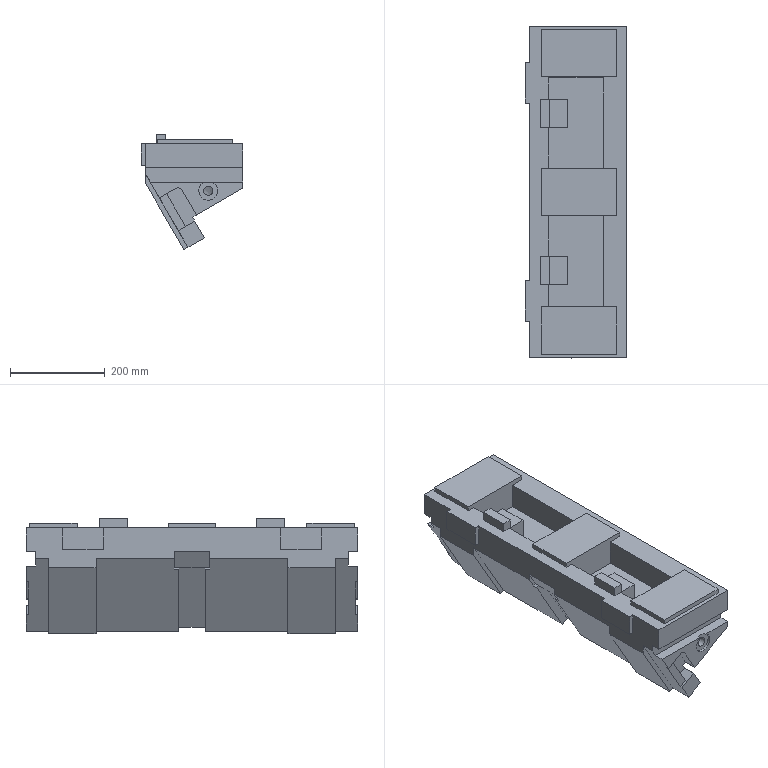Part | NX | features solid 2 | 1 solid | 108 faces | box 215 x 700 x 243.363 mm | volume 18215723 mm3 | plane 96 | cylinder 10 | cone 2 | commonest cylinder face diameters 20 x8 40 x2